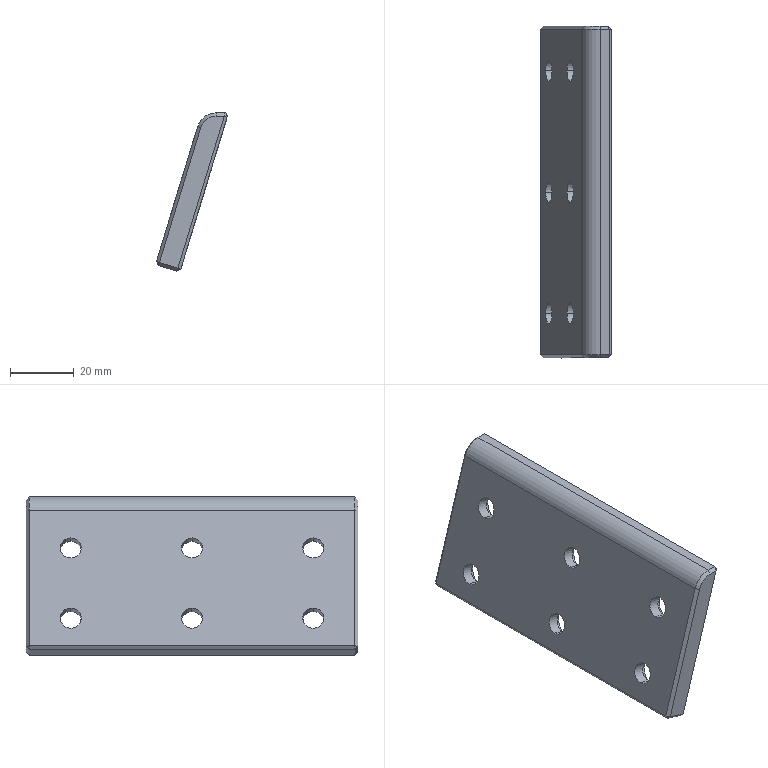Part | Creo | 1 solid | 74 faces | box 22.323 x 104 x 49.611 mm | volume 38395 mm3 | cone 26 | cylinder 25 | plane 23 | commonest cylinder face diameters 6.6 x12 13 x12 12 x1